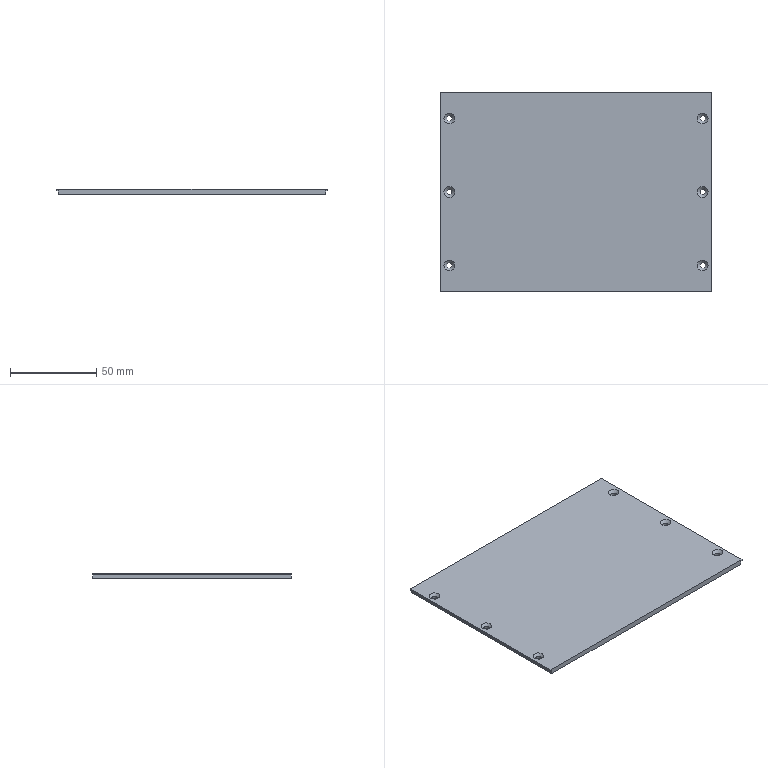NC program | NX | posted by the shop | part box 156.6 x 115 x 3 mm
Whole program:
%
(CUTTING TIME: 6.52)
(NAME: 3953270)
G17 G40 G49 G80 G90
G91 G28 Z0.
(TOOL_NAME :T3-D10-CX )
T03 M06
G00 G90 G54 X-84.3 Y63.009 S6500 M03
G43 Z100. H03 M08 T04
G01 X-84.3 Y63.009 Z-3.5 F5000.
G41 X-83.8 Y63. F1500. D03
X-78.3 Y63.
X78.3 Y63.
X83.8 Y63.
G40 X84.3 Y63.009
G00 Z50.
G01 X84.3 Y-63.009 F5000.
X84.3 Y-63.009 Z-3.5
G41 X83.8 Y-63. F1500.
X78.3 Y-63.
X-78.3 Y-63.
X-83.8 Y-63.
G40 X-84.3 Y-63.009
G00 Z100.
M05
M09
G91 G28 Z0.
M01
(TOOL_NAME :T4-D10-JX )
T04 M06
G00 G90 G54 X-84.3 Y62.509 S6500 M03
G43 Z100. H04 M08 T10
G01 X-84.3 Y62.509 Z-3.5 F5000.
G41 X-83.8 Y62.5 F1500. D04
X-78.3 Y62.5
X78.3 Y62.5
X83.8 Y62.5
G40 X84.3 Y62.509
G00 Z50.
G01 X84.3 Y-62.509 F5000.
X84.3 Y-62.509 Z-3.5
G41 X83.8 Y-62.5 F1500.
X78.3 Y-62.5
X-78.3 Y-62.5
X-83.8 Y-62.5
G40 X-84.3 Y-62.509
G00 Z100.
M05
M09
G91 G28 Z0.
M01
(TOOL_NAME :T10-D4-90度 )
T10 M06
G00 G90 G54 X-81. Y58.509 S6500 M03
G43 Z100. H10 M08 T03
G01 X-81. Y58.509 Z-1. F5000.
G41 X-80.5 Y58.5 F1500.
X-78.3 Y58.5
X78.3 Y58.5
X80.5 Y58.5
G40 X81. Y58.509
G00 Z50.
G01 X81. Y-58.509 F5000.
X81. Y-58.509 Z-1.
G41 X80.5 Y-58.5 F1500.
X78.3 Y-58.5
X-78.3 Y-58.5
X-80.5 Y-58.5
G40 X-81. Y-58.509
G00 Z100.
M05
M09
G91 G28 Z0.
M01
M00 （ 换压板）
(TOOL_NAME :T3-D10-CX )
T03 M06
G00 G90 G54 X-82.609 Y-63.5 S6500 M03
G43 Z100. H03 M08 T04
G01 X-82.609 Y-63.5 Z-1.8 F5000.
G41 X-82.6 Y-63. F1500. D03
X-82.6 Y-57.5
X-82.6 Y57.5
X-82.6 Y63.
G40 X-82.609 Y63.5
G00 Z50.
G01 X82.609 Y63.5 F5000.
X82.609 Y63.5 Z-1.8
G41 X82.6 Y63. F1500.
X82.6 Y57.5
X82.6 Y-57.5
X82.6 Y-63.
G40 X82.609 Y-63.5
G00 Z100.
G00 G90 G54 X83.609 Y63.5 S6500 M03
G01 X83.609 Y63.5 Z-3.5 F5000.
G41 X83.6 Y63. F1500.
X83.6 Y57.5
X83.6 Y-57.5
X83.6 Y-63.
G40 X83.609 Y-63.5
G00 Z50.
G01 X-83.609 Y-63.5 F5000.
X-83.609 Y-63.5 Z-3.5
G41 X-83.6 Y-63. F1500.
X-83.6 Y-57.5
X-83.6 Y57.5
X-83.6 Y63.
G40 X-83.609 Y63.5
G00 Z100.
G00 Z103.
G90 G54 X47.462 Y-2.134 S6500 M03
G01 X47.462 Y-2.134 Z3. F5000.
G03 X47.462 Y-2.134 Z2.506 I-3.962 J2.134 F2500.
X47.462 Y-2.134 Z2.013 I-3.962 J2.134
X47.462 Y-2.134 Z1.519 I-3.962 J2.134
X47.462 Y-2.134 Z1.026 I-3.962 J2.134
X47.462 Y-2.134 Z.532 I-3.962 J2.134
X47.462 Y-2.134 Z.039 I-3.962 J2.134
X48. Y0.0 Z0.0 I-3.962 J2.134
G01 X48. Y5.31
X50.403 Y9.812
X48. Y5.31
X40.074 Y0.0
X48. Y-5.31
X50.403 Y-9.812
X48. Y-5.31
X48. Y0.0
X55.5 Y0.0
X55.5 Y19.363
X57.903 Y23.864
X55.5 Y19.363
X26.6 Y0.0
X55.5 Y-19.363
X57.903 Y-23.864
X55.5 Y-19.363
X55.5 Y0.0
X63. Y0.0
X63. Y33.416
X13.126 Y0.0
X63. Y-33.416
X63. Y0.0
G00 Z103.
G90 G54 X-2.134 Y-29.662
G01 X-2.134 Y-29.662 Z3. F5000.
G03 X-2.134 Y-29.662 Z2.506 I2.134 J3.962 F2500.
X-2.134 Y-29.662 Z2.013 I2.134 J3.962
X-2.134 Y-29.662 Z1.519 I2.134 J3.962
X-2.134 Y-29.662 Z1.026 I2.134 J3.962
X-2.134 Y-29.662 Z.532 I2.134 J3.962
X-2.134 Y-29.662 Z.039 I2.134 J3.962
X0.0 Y-30.2 Z0.0 I2.134 J3.962
G01 X8.615 Y-30.2
X0.0 Y-24.428
X-8.615 Y-30.2
X0.0 Y-30.2
X0.0 Y-34.7
X23.416 Y-34.7
X29.319 Y-36.495
X23.416 Y-34.7
X0.0 Y-19.011
X-23.416 Y-34.7
X-29.319 Y-36.495
X-23.416 Y-34.7
X0.0 Y-34.7
X0.0 Y-42.2
X48.085 Y-42.2
X0.0 Y-9.984
X-48.085 Y-42.2
X0.0 Y-42.2
G00 Z103.
G90 G54 X-47.462 Y2.134
G01 X-47.462 Y2.134 Z3. F5000.
G03 X-47.462 Y2.134 Z2.506 I3.962 J-2.134 F2500.
X-47.462 Y2.134 Z2.013 I3.962 J-2.134
X-47.462 Y2.134 Z1.519 I3.962 J-2.134
X-47.462 Y2.134 Z1.026 I3.962 J-2.134
X-47.462 Y2.134 Z.532 I3.962 J-2.134
X-47.462 Y2.134 Z.039 I3.962 J-2.134
X-48. Y0.0 Z0.0 I3.962 J-2.134
G01 X-48. Y-5.31
X-50.403 Y-9.812
X-48. Y-5.31
X-40.074 Y0.0
X-48. Y5.31
X-50.403 Y9.812
X-48. Y5.31
X-48. Y0.0
X-55.5 Y0.0
X-55.5 Y-19.363
X-57.903 Y-23.864
X-55.5 Y-19.363
X-26.6 Y0.0
X-55.5 Y19.363
X-57.903 Y23.864
X-55.5 Y19.363
X-55.5 Y0.0
X-63. Y0.0
X-63. Y-33.416
X-13.126 Y0.0
X-63. Y33.416
X-63. Y0.0
G00 Z103.
G90 G54 X2.134 Y29.662
G01 X2.134 Y29.662 Z3. F5000.
G03 X2.134 Y29.662 Z2.506 I-2.134 J-3.962 F2500.
X2.134 Y29.662 Z2.013 I-2.134 J-3.962
X2.134 Y29.662 Z1.519 I-2.134 J-3.962
X2.134 Y29.662 Z1.026 I-2.134 J-3.962
X2.134 Y29.662 Z.532 I-2.134 J-3.962
X2.134 Y29.662 Z.039 I-2.134 J-3.962
X0.0 Y30.2 Z0.0 I-2.134 J-3.962
G01 X-8.615 Y30.2
X0.0 Y24.428
X8.615 Y30.2
X0.0 Y30.2
X0.0 Y34.7
X-23.416 Y34.7
X-29.319 Y36.495
X-23.416 Y34.7
X0.0 Y19.011
X23.416 Y34.7
X29.319 Y36.495
X23.416 Y34.7
X0.0 Y34.7
X0.0 Y42.2
X-48.085 Y42.2
X0.0 Y9.984
X48.085 Y42.2
X0.0 Y42.2
G00 Z103.
M05
M09
G91 G28 Z0.
M01
(TOOL_NAME :T4-D10-JX )
T04 M06
G00 G90 G54 X-82.309 Y-63.5 S6500 M03
G43 Z100. H04 M08 T06
G01 X-82.309 Y-63.5 Z-2.1 F5000.
G41 X-82.3 Y-63. F1500. D04
X-82.3 Y-57.5
X-82.3 Y57.5
X-82.3 Y63.
G40 X-82.309 Y63.5
G00 Z50.
G01 X82.309 Y63.5 F5000.
X82.309 Y63.5 Z-2.1
G41 X82.3 Y63. F1500.
X82.3 Y57.5
X82.3 Y-57.5
X82.3 Y-63.
G40 X82.309 Y-63.5
G00 Z100.
G00 G90 G54 X83.309 Y63.5 S6500 M03
G01 X83.309 Y63.5 Z-3.5 F5000.
G41 X83.3 Y63. F1500.
X83.3 Y57.5
X83.3 Y-57.5
X83.3 Y-63.
G40 X83.309 Y-63.5
G00 Z50.
G01 X-83.309 Y-63.5 F5000.
X-83.309 Y-63.5 Z-3.5
G41 X-83.3 Y-63. F1500.
X-83.3 Y-57.5
X-83.3 Y57.5
X-83.3 Y63.
G40 X-83.309 Y63.5
G00 Z100.
M05
M09
G91 G28 Z0.
M01
(TOOL_NAME :T6-D8-JX )
T06 M06
G00 G90 G54 X41.021 Y-2.162 S6500 M03
G43 Z103. H06 M08 T10
G01 X41.021 Y-2.162 Z3. F5000.
G03 X41.021 Y-2.162 Z2.605 I2.879 J2.162 F2500.
X41.021 Y-2.162 Z2.21 I2.879 J2.162
X41.021 Y-2.162 Z1.816 I2.879 J2.162
X41.021 Y-2.162 Z1.421 I2.879 J2.162
X41.021 Y-2.162 Z1.026 I2.879 J2.162
X41.021 Y-2.162 Z.631 I2.879 J2.162
X41.021 Y-2.162 Z.236 I2.879 J2.162
X41.021 Y-2.162 Z-.159 I2.879 J2.162
X41.021 Y-2.162 Z-.553 I2.879 J2.162
X41.021 Y-2.162 Z-.948 I2.879 J2.162
X41.021 Y-2.162 Z-1.343 I2.879 J2.162
X47.5 Y0.0 Z-1.5 I2.879 J2.162
G01 X47.5 Y4.373
X40.973 Y0.0
X47.5 Y-4.373
X47.5 Y0.0
X50.3 Y0.0
X50.3 Y9.62
X35.942 Y0.0
X50.3 Y-9.62
X50.3 Y0.0
X53.1 Y0.0
X53.1 Y14.866
X30.912 Y0.0
X53.1 Y-14.866
X53.1 Y0.0
X55.9 Y0.0
X55.9 Y20.112
X25.881 Y0.0
X55.9 Y-20.112
X55.9 Y0.0
X58.7 Y0.0
X58.7 Y25.359
X20.851 Y0.0
X58.7 Y-25.359
X58.7 Y0.0
X61.5 Y0.0
X61.5 Y30.605
X15.821 Y0.0
X61.5 Y-30.605
X61.5 Y0.0
X64.3 Y0.0
X64.3 Y33.978
G03 X62.743 Y34.808 I-1. J0.0
G01 X12.03 Y.831
G03 X12.03 Y-.831 I.557 J-.831
G01 X62.743 Y-34.808
G03 X64.3 Y-33.978 I.557 J.831
G01 X64.3 Y0.0
G00 Z103.
G90 G54 X2.162 Y23.021
G01 X2.162 Y23.021 Z3. F5000.
G03 X2.162 Y23.021 Z2.605 I-2.162 J2.879 F2500.
X2.162 Y23.021 Z2.21 I-2.162 J2.879
X2.162 Y23.021 Z1.816 I-2.162 J2.879
X2.162 Y23.021 Z1.421 I-2.162 J2.879
X2.162 Y23.021 Z1.026 I-2.162 J2.879
X2.162 Y23.021 Z.631 I-2.162 J2.879
X2.162 Y23.021 Z.236 I-2.162 J2.879
X2.162 Y23.021 Z-.159 I-2.162 J2.879
X2.162 Y23.021 Z-.553 I-2.162 J2.879
X2.162 Y23.021 Z-.948 I-2.162 J2.879
X2.162 Y23.021 Z-1.343 I-2.162 J2.879
X0.0 Y29.5 Z-1.5 I-2.162 J2.879
G01 X-6.313 Y29.5
X0.0 Y25.271
X6.313 Y29.5
X0.0 Y29.5
X0.0 Y32.3
X-15.522 Y32.3
X0.0 Y21.9
X15.522 Y32.3
X0.0 Y32.3
X0.0 Y35.1
X-24.732 Y35.1
X0.0 Y18.53
X24.732 Y35.1
X0.0 Y35.1
X0.0 Y37.9
X-33.941 Y37.9
X0.0 Y15.159
X33.941 Y37.9
X0.0 Y37.9
X0.0 Y40.7
X-43.151 Y40.7
X0.0 Y11.789
X43.151 Y40.7
X0.0 Y40.7
X0.0 Y43.5
X-49.071 Y43.5
G03 X-49.628 Y41.669 I0.0 J-1.
G01 X-.557 Y8.792
G03 X.557 Y8.792 I.557 J.831
G01 X49.628 Y41.669
G03 X49.071 Y43.5 I-.557 J.831
G01 X0.0 Y43.5
G00 Z103.
G90 G54 X-41.021 Y2.162
G01 X-41.021 Y2.162 Z3. F5000.
G03 X-41.021 Y2.162 Z2.605 I-2.879 J-2.162 F2500.
X-41.021 Y2.162 Z2.21 I-2.879 J-2.162
X-41.021 Y2.162 Z1.816 I-2.879 J-2.162
X-41.021 Y2.162 Z1.421 I-2.879 J-2.162
X-41.021 Y2.162 Z1.026 I-2.879 J-2.162
X-41.021 Y2.162 Z.631 I-2.879 J-2.162
X-41.021 Y2.162 Z.236 I-2.879 J-2.162
X-41.021 Y2.162 Z-.159 I-2.879 J-2.162
X-41.021 Y2.162 Z-.553 I-2.879 J-2.162
X-41.021 Y2.162 Z-.948 I-2.879 J-2.162
X-41.021 Y2.162 Z-1.343 I-2.879 J-2.162
X-47.5 Y0.0 Z-1.5 I-2.879 J-2.162
G01 X-47.5 Y-4.373
X-40.973 Y0.0
X-47.5 Y4.373
X-47.5 Y0.0
X-50.3 Y0.0
X-50.3 Y-9.62
X-35.942 Y0.0
X-50.3 Y9.62
X-50.3 Y0.0
X-53.1 Y0.0
X-53.1 Y-14.866
X-30.912 Y0.0
X-53.1 Y14.866
X-53.1 Y0.0
X-55.9 Y0.0
X-55.9 Y-20.112
X-25.881 Y0.0
X-55.9 Y20.112
X-55.9 Y0.0
X-58.7 Y0.0
X-58.7 Y-25.359
X-20.851 Y0.0
X-58.7 Y25.359
X-58.7 Y0.0
X-61.5 Y0.0
X-61.5 Y-30.605
X-15.821 Y0.0
X-61.5 Y30.605
X-61.5 Y0.0
X-64.3 Y0.0
X-64.3 Y-33.978
G03 X-62.743 Y-34.808 I1. J0.0
G01 X-12.03 Y-.831
G03 X-12.03 Y.831 I-.557 J.831
G01 X-62.743 Y34.808
G03 X-64.3 Y33.978 I-.557 J-.831
G01 X-64.3 Y0.0
G00 Z103.
G90 G54 X-2.162 Y-23.021
G01 X-2.162 Y-23.021 Z3. F5000.
G03 X-2.162 Y-23.021 Z2.605 I2.162 J-2.879 F2500.
X-2.162 Y-23.021 Z2.21 I2.162 J-2.879
X-2.162 Y-23.021 Z1.816 I2.162 J-2.879
X-2.162 Y-23.021 Z1.421 I2.162 J-2.879
X-2.162 Y-23.021 Z1.026 I2.162 J-2.879
X-2.162 Y-23.021 Z.631 I2.162 J-2.879
X-2.162 Y-23.021 Z.236 I2.162 J-2.879
X-2.162 Y-23.021 Z-.159 I2.162 J-2.879
X-2.162 Y-23.021 Z-.553 I2.162 J-2.879
X-2.162 Y-23.021 Z-.948 I2.162 J-2.879
X-2.162 Y-23.021 Z-1.343 I2.162 J-2.879
X0.0 Y-29.5 Z-1.5 I2.162 J-2.879
G01 X6.313 Y-29.5
X0.0 Y-25.271
X-6.313 Y-29.5
X0.0 Y-29.5
X0.0 Y-32.3
X15.522 Y-32.3
X0.0 Y-21.9
X-15.522 Y-32.3
X0.0 Y-32.3
X0.0 Y-35.1
X24.732 Y-35.1
X0.0 Y-18.53
X-24.732 Y-35.1
X0.0 Y-35.1
X0.0 Y-37.9
X33.941 Y-37.9
X0.0 Y-15.159
X-33.941 Y-37.9
X0.0 Y-37.9
X0.0 Y-40.7
X43.151 Y-40.7
X0.0 Y-11.789
X-43.151 Y-40.7
X0.0 Y-40.7
X0.0 Y-43.5
X49.071 Y-43.5
G03 X49.628 Y-41.669 I0.0 J1.
G01 X.557 Y-8.792
G03 X-.557 Y-8.792 I-.557 J-.831
G01 X-49.628 Y-41.669
G03 X-49.071 Y-43.5 I.557 J-.831
G01 X0.0 Y-43.5
G00 Z103.
M05
M09
G91 G28 Z0.
M01
(TOOL_NAME :T10-D4-90度 )
T10 M06
G00 G90 G54 X50.073 Y41.005 S6500 M03
G43 Z100. H10 M08 T13
G01 X50.073 Y41.005 Z-1. F5000.
G41 X51.298 Y39.177 F1500.
G03 X49.071 Y46.5 I-2.226 J3.323
G01 X-49.071 Y46.5
G03 X-51.298 Y39.177 I0.0 J-4.
G01 X-2.226 Y6.299
G03 X2.226 Y6.299 I2.226 J3.323
G01 X51.298 Y39.177
G03 X51.461 Y39.292 I-2.226 J3.323
G40 G01 X50.147 Y41.057
G00 Z100.
G90 G54 X-65.1 Y-33.978
G01 X-65.1 Y-33.978 Z-1. F5000.
G41 X-67.3 Y-33.978 F1500.
G03 X-61.074 Y-37.301 I4. J0.0
G01 X-10.36 Y-3.323
G03 X-10.36 Y3.323 I-2.226 J3.323
G01 X-61.074 Y37.301
G03 X-67.3 Y33.978 I-2.226 J-3.323
G01 X-67.3 Y-33.978
G03 X-67.295 Y-34.178 I4. J0.0
G40 G01 X-65.098 Y-34.068
G00 Z100.
G90 G54 X-50.073 Y-41.005
G01 X-50.073 Y-41.005 Z-1. F5000.
G41 X-51.298 Y-39.177 F1500.
G03 X-49.071 Y-46.5 I2.226 J-3.323
G01 X49.071 Y-46.5
G03 X51.298 Y-39.177 I0.0 J4.
G01 X2.226 Y-6.299
G03 X-2.226 Y-6.299 I-2.226 J-3.323
G01 X-51.298 Y-39.177
G03 X-51.461 Y-39.292 I2.226 J-3.323
G40 G01 X-50.147 Y-41.057
G00 Z100.
G90 G54 X62.298 Y-35.473
G01 X62.298 Y-35.473 Z-1. F5000.
G41 X61.074 Y-37.301 F1500.
G03 X67.3 Y-33.978 I2.226 J3.323
G01 X67.3 Y33.978
G03 X61.074 Y37.301 I-4. J0.0
G01 X10.36 Y3.323
G03 X10.36 Y-3.323 I2.226 J-3.323
G01 X61.074 Y-37.301
G03 X61.242 Y-37.408 I2.226 J3.323
G40 G01 X62.374 Y-35.521
G00 Z100.
G00 G90 G54 X79.609 Y60.2 S6500 M03
G01 X79.609 Y60.2 Z-3.1 F5000.
G41 X79.6 Y59.7 F1500.
X79.6 Y57.5
X79.6 Y-57.5
X79.6 Y-59.7
G40 X79.609 Y-60.2
G00 Z47.9
G01 X-79.609 Y-60.2 F5000.
X-79.609 Y-60.2 Z-3.1
G41 X-79.6 Y-59.7 F1500.
X-79.6 Y-57.5
X-79.6 Y57.5
X-79.6 Y59.7
G40 X-79.609 Y60.2
G00 Z100.
G00 G90 G54 X78.309 Y60.2 S6500 M03
G01 X78.309 Y60.2 Z-1. F5000.
G41 X78.3 Y59.7 F1500.
X78.3 Y57.5
X78.3 Y-57.5
X78.3 Y-59.7
G40 X78.309 Y-60.2
G00 Z50.
G01 X-78.309 Y-60.2 F5000.
X-78.309 Y-60.2 Z-1.
G41 X-78.3 Y-59.7 F1500.
X-78.3 Y-57.5
X-78.3 Y57.5
X-78.3 Y59.7
G40 X-78.309 Y60.2
G00 Z100.
G00 G90 G54 X73.3 Y-42.5 S1200 M03
Z50.
G98 G83 X73.3 Y-42.5 Z-.5 R1.5 F100. Q2.
X73.3 Y0.0
X73.3 Y42.5
X-73.3 Y42.5
X-73.3 Y0.0
X-73.3 Y-42.5
G80
G00 Z50.
M05
M09
G91 G28 Z0.
M01
(TOOL_NAME :T13-ZT3.2 )
T13 M06
G00 G90 G54 X73.3 Y-42.5 S1200 M03
G43 Z50. H13 M08 T03
G98 G83 X73.3 Y-42.5 Z-5. R1.5 F100. Q2.
X73.3 Y0.0
X73.3 Y42.5
X-73.3 Y42.5
X-73.3 Y0.0
X-73.3 Y-42.5
G80
G00 Z50.
M05
M09
G91 G28 Z0.
G91 G28 Y0.
M30
%